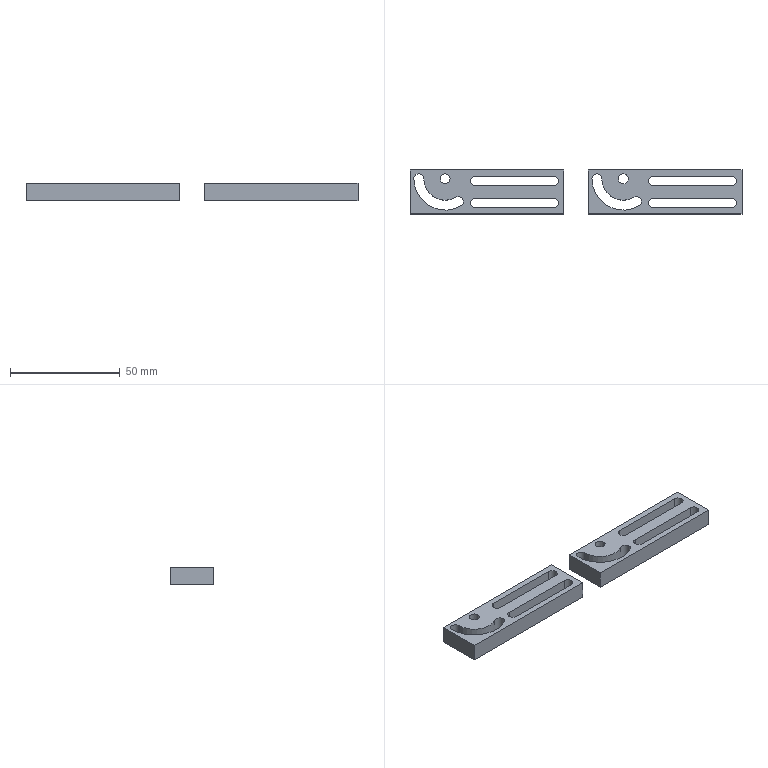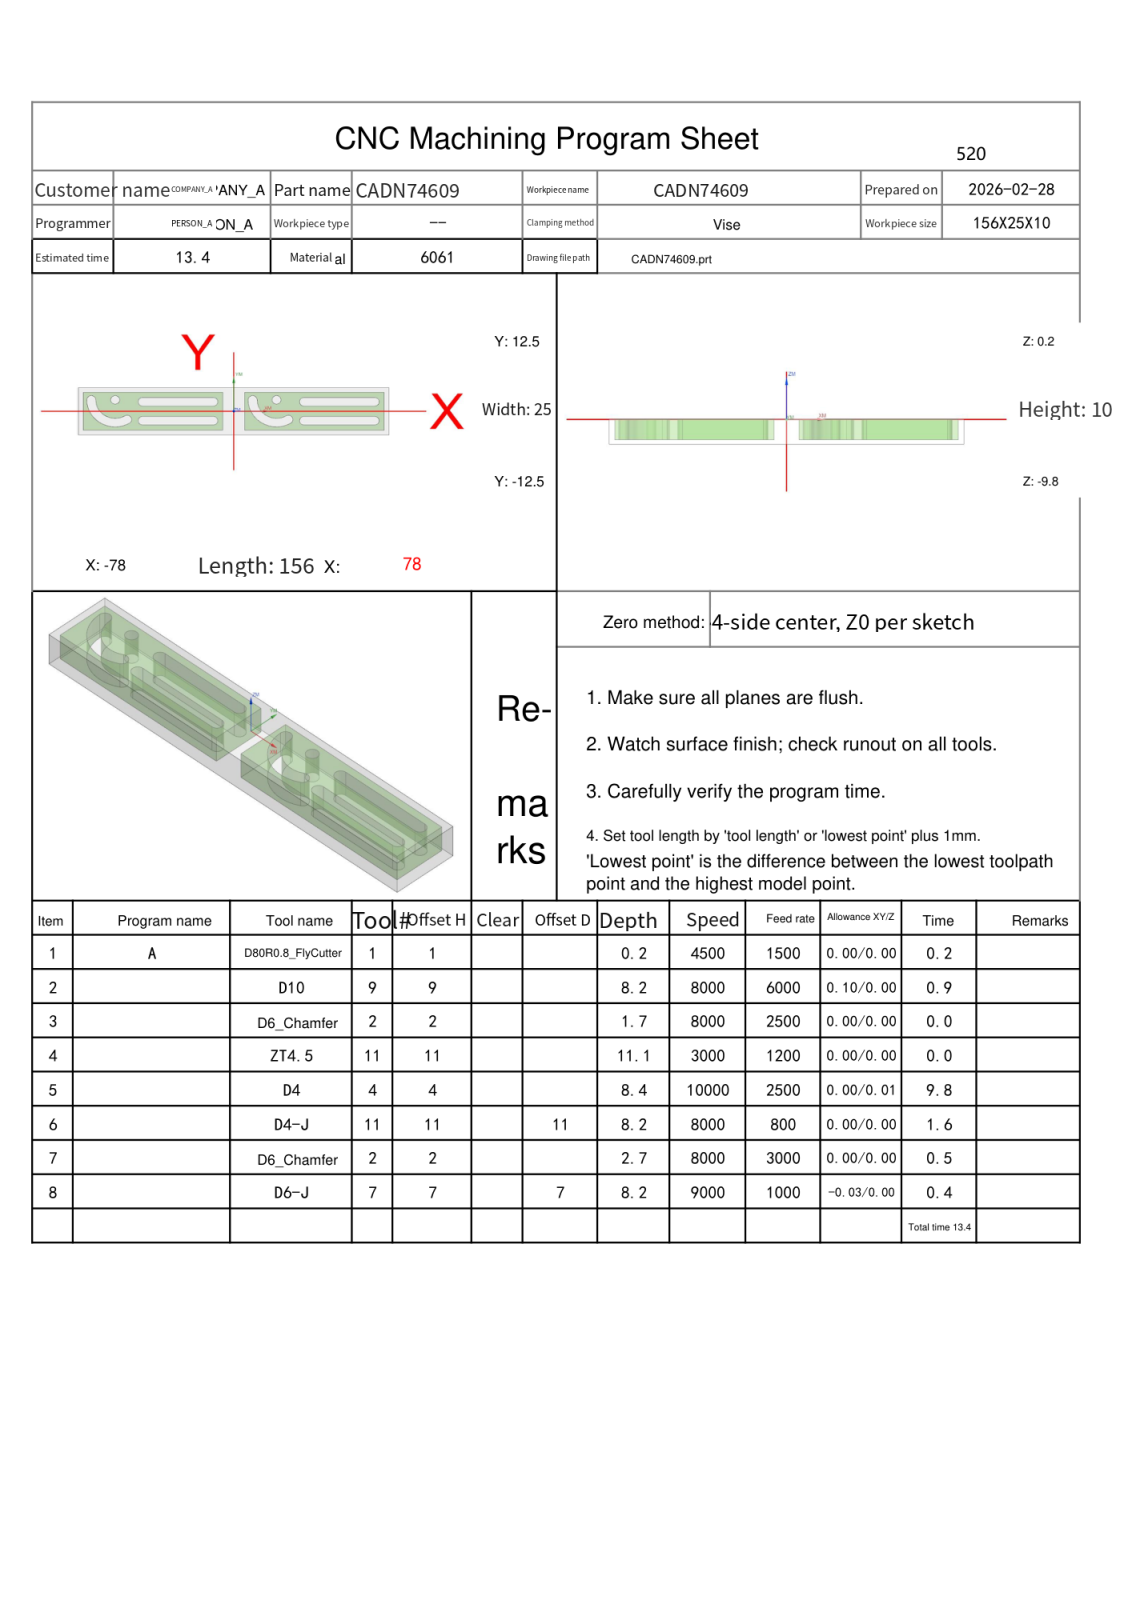NC program | NX | posted by the shop | part box 151 x 20 x 8 mm
Lines 3238 to 3746 of 3746:
N6 T11 M06
(D4-J  D=4. R=0. H=11 ce=0.00 di=0.00)
G00 G90 G54 X-28.2 Y5. M03 S8000
G43 H11 Z50.
M08
Z-3.5
G01 Z-4. F500.
G41 D11
Y4.95
G03 X-28. Y4.75 I.2 J0.0
G01 X-10.25
G03 X-10. Y5. I0.0 J.25
X-10.25 Y5.25 I-.25 J0.0
G01 X-45.75
G03 X-46. Y5. I0.0 J-.25
X-45.75 Y4.75 I.25 J0.0
G01 X-28.
X-27.5
G03 X-27.3 Y4.95 I0.0 J.2
G01 G40 Y5.
Z-3.5
G00 Z1.
X-28.2
Z-7.5
G01 Z-8.
G41 D11
Y4.95
G03 X-28. Y4.75 I.2 J0.0
G01 X-10.25
G03 X-10. Y5. I0.0 J.25
X-10.25 Y5.25 I-.25 J0.0
G01 X-45.75
G03 X-46. Y5. I0.0 J-.25
X-45.75 Y4.75 I.25 J0.0
G01 X-28.
X-27.5
G03 X-27.3 Y4.95 I0.0 J.2
G01 G40 Y5.
Z-7.5
G00 Z50.
X-27.8 Y-5.
Z-3.5
G01 Z-4.
G41 D11
Y-4.95
G03 X-28. Y-4.75 I-.2 J0.0
G01 X-45.75
G03 X-46. Y-5. I0.0 J-.25
X-45.75 Y-5.25 I.25 J0.0
G01 X-10.25
G03 X-10. Y-5. I0.0 J.25
X-10.25 Y-4.75 I-.25 J0.0
G01 X-28.
X-28.5
G03 X-28.7 Y-4.95 I0.0 J-.2
G01 G40 Y-5.
Z-3.5
G00 Z1.
X-27.8
Z-7.5
G01 Z-8.
G41 D11
Y-4.95
G03 X-28. Y-4.75 I-.2 J0.0
G01 X-45.75
G03 X-46. Y-5. I0.0 J-.25
X-45.75 Y-5.25 I.25 J0.0
G01 X-10.25
G03 X-10. Y-5. I0.0 J.25
X-10.25 Y-4.75 I-.25 J0.0
G01 X-28.
X-28.5
G03 X-28.7 Y-4.95 I0.0 J-.2
G01 G40 Y-5.
Z-7.5
G00 Z50.
X52.8 Y5.
Z-3.5
G01 Z-4.
G41 D11
Y4.95
G03 X53. Y4.75 I.2 J0.0
G01 X70.75
G03 X71. Y5. I0.0 J.25
X70.75 Y5.25 I-.25 J0.0
G01 X35.25
G03 X35. Y5. I0.0 J-.25
X35.25 Y4.75 I.25 J0.0
G01 X53.
X53.5
G03 X53.7 Y4.95 I0.0 J.2
G01 G40 Y5.
Z-3.5
G00 Z1.
X52.8
Z-7.5
G01 Z-8.
G41 D11
Y4.95
G03 X53. Y4.75 I.2 J0.0
G01 X70.75
G03 X71. Y5. I0.0 J.25
X70.75 Y5.25 I-.25 J0.0
G01 X35.25
G03 X35. Y5. I0.0 J-.25
X35.25 Y4.75 I.25 J0.0
G01 X53.
X53.5
G03 X53.7 Y4.95 I0.0 J.2
G01 G40 Y5.
Z-7.5
G00 Z50.
X53.2 Y-5.
Z-3.5
G01 Z-4.
G41 D11
Y-4.95
G03 X53. Y-4.75 I-.2 J0.0
G01 X35.25
G03 X35. Y-5. I0.0 J-.25
X35.25 Y-5.25 I.25 J0.0
G01 X70.75
G03 X71. Y-5. I0.0 J.25
X70.75 Y-4.75 I-.25 J0.0
G01 X53.
X52.5
G03 X52.3 Y-4.95 I0.0 J-.2
G01 G40 Y-5.
Z-3.5
G00 Z1.
X53.2
Z-7.5
G01 Z-8.
G41 D11
Y-4.95
G03 X53. Y-4.75 I-.2 J0.0
G01 X35.25
G03 X35. Y-5. I0.0 J-.25
X35.25 Y-5.25 I.25 J0.0
G01 X70.75
G03 X71. Y-5. I0.0 J.25
X70.75 Y-4.75 I-.25 J0.0
G01 X53.
X52.5
G03 X52.3 Y-4.95 I0.0 J-.2
G01 G40 Y-5.
Z-7.5
G00 Z50.
G00 G90 X15.328 Y-4.291 M03 S8000
Z50.
Z-3.5
G01 Z-4. F800.
G41 D11
X15.302 Y-4.336
X15.275 Y-4.436
G03 X15.375 Y-4.609 I.2 J0.0
X21.5 Y-6.25 I6.125 J10.609
X27.625 Y-4.609 I0.0 J12.25
X27.75 Y-4.392 I-.125 J.217
X27.5 Y-4.142 I-.25 J0.0
G01 X27.375 Y-4.176
G02 X21.5 Y-5.75 I-5.875 J10.176
X9.75 Y6. I0.0 J11.75
G03 X9.5 Y6.25 I-.25 J0.0
X9.25 Y6. I0.0 J-.25
X15.375 Y-4.609 I12.25 J0.0
X15.813 Y-4.85 I6.125 J10.609
G01 X15.906 Y-4.873
G03 X16.084 Y-4.764 I0.0 J.2
G01 G40 X16.107 Y-4.72
Z-3.5
G00 Z1.
X15.328 Y-4.291
Z-7.5
G01 Z-8.
G41 D11
X15.302 Y-4.336
X15.275 Y-4.436
G03 X15.375 Y-4.609 I.2 J0.0
X21.5 Y-6.25 I6.125 J10.609
X27.625 Y-4.609 I0.0 J12.25
X27.75 Y-4.392 I-.125 J.217
X27.5 Y-4.142 I-.25 J0.0
G01 X27.375 Y-4.176
G02 X21.5 Y-5.75 I-5.875 J10.176
X9.75 Y6. I0.0 J11.75
G03 X9.5 Y6.25 I-.25 J0.0
X9.25 Y6. I0.0 J-.25
X15.375 Y-4.609 I12.25 J0.0
X15.813 Y-4.85 I6.125 J10.609
G01 X15.906 Y-4.873
G03 X16.084 Y-4.764 I0.0 J.2
G01 G40 X16.107 Y-4.72
Z-7.5
G00 Z50.
X-65.672 Y-4.291
Z-3.5
G01 Z-4.
G41 D11
X-65.698 Y-4.336
X-65.725 Y-4.436
G03 X-65.625 Y-4.609 I.2 J0.0
X-59.5 Y-6.25 I6.125 J10.609
X-53.375 Y-4.609 I0.0 J12.25
X-53.25 Y-4.392 I-.125 J.217
X-53.5 Y-4.142 I-.25 J0.0
G01 X-53.625 Y-4.176
G02 X-59.5 Y-5.75 I-5.875 J10.176
X-71.25 Y6. I0.0 J11.75
G03 X-71.5 Y6.25 I-.25 J0.0
X-71.75 Y6. I0.0 J-.25
X-65.625 Y-4.609 I12.25 J0.0
X-65.187 Y-4.85 I6.125 J10.609
G01 X-65.094 Y-4.873
G03 X-64.916 Y-4.764 I0.0 J.2
G01 G40 X-64.893 Y-4.72
Z-3.5
G00 Z1.
X-65.672 Y-4.291
Z-7.5
G01 Z-8.
G41 D11
X-65.698 Y-4.336
X-65.725 Y-4.436
G03 X-65.625 Y-4.609 I.2 J0.0
X-59.5 Y-6.25 I6.125 J10.609
X-53.375 Y-4.609 I0.0 J12.25
X-53.25 Y-4.392 I-.125 J.217
X-53.5 Y-4.142 I-.25 J0.0
G01 X-53.625 Y-4.176
G02 X-59.5 Y-5.75 I-5.875 J10.176
X-71.25 Y6. I0.0 J11.75
G03 X-71.5 Y6.25 I-.25 J0.0
X-71.75 Y6. I0.0 J-.25
X-65.625 Y-4.609 I12.25 J0.0
X-65.187 Y-4.85 I6.125 J10.609
G01 X-65.094 Y-4.873
G03 X-64.916 Y-4.764 I0.0 J.2
G01 G40 X-64.893 Y-4.72
Z-7.5
G00 Z50.
G91 G28 Z0.0
M05
M09
G91 G28 Z0.0
M01
N7 T02 M06
(D6_Chamfer  D=6. R=0. H=02 ce=0.00 di=0.00)
G00 G90 G54 X-40.25 Y-12.128 M03 S8000
G43 H02 Z50.
M08
Z2.099
G01 Z-1.5 F3000.
G03 X-40.17 Y-11.828 I-.52 J.3
X-40.47 Y-11.308 I-.6 J0.0
G01 X-40.5 Y-11.3
X-75.5
G02 X-76.8 Y-10. I0.0 J1.3
G01 Y10.
G02 X-75.5 Y11.3 I1.3 J0.0
G01 X-5.5
G02 X-4.2 Y10. I0.0 J-1.3
G01 Y-10.
G02 X-5.5 Y-11.3 I-1.3 J0.0
G01 X-40.5
X-40.53 Y-11.308
G03 X-40.83 Y-11.828 I.3 J-.52
X-40.75 Y-12.128 I.6 J0.0
G01 Z2.099
G00 Z50.
X-65.809 Y-4.367
Z2.121
G01 Z-1.5
G03 X-66.09 Y-4.875 I.319 J-.508
X-65.998 Y-5.194 I.6 J0.0
G01 X-65.975 Y-5.215
G03 X-59.5 Y-6.95 I6.475 J11.215
X-53.025 Y-5.215 I0.0 J12.95
X-52.55 Y-4.392 I-.475 J.823
X-53.025 Y-3.57 I-.95 J0.0
G01 X-53.254 Y-3.475
X-53.5 Y-3.442
X-53.746 Y-3.475
X-53.975 Y-3.57
G02 X-59.5 Y-5.05 I-5.525 J9.57
X-70.55 Y6. I0.0 J11.05
G03 X-71.5 Y6.95 I-.95 J0.0
X-71.975 Y6.823 I0.0 J-.95
G01 X-72.172 Y6.672
X-72.323 Y6.475
X-72.418 Y6.246
X-72.45 Y6.
G03 X-65.975 Y-5.215 I12.95 J0.0
G01 X-65.945 Y-5.224
X-65.923 Y-5.225
G03 X-65.323 Y-4.647 I0.0 J.6
G01 Z2.121
G00 Z50.
X-28.25 Y-5.122
Z2.099
G01 Z-1.5
G03 X-28.33 Y-5.422 I.52 J-.3
X-28.03 Y-5.942 I.6 J0.0
G01 X-28. Y-5.95
X-10.25
G03 X-9.3 Y-5. I0.0 J.95
X-9.427 Y-4.525 I-.95 J0.0
G01 X-9.578 Y-4.328
X-9.775 Y-4.177
X-10.004 Y-4.082
X-10.25 Y-4.05
X-45.75
G03 X-46.7 Y-5. I0.0 J-.95
X-46.573 Y-5.475 I.95 J0.0
G01 X-46.422 Y-5.672
X-46.225 Y-5.823
X-45.996 Y-5.918
X-45.75 Y-5.95
X-28.
X-27.97 Y-5.942
G03 X-27.67 Y-5.422 I-.3 J.52
X-27.75 Y-5.122 I-.6 J0.0
G01 Z2.099
G00 Z6.
X-28.25 Y4.878
Z2.099
G01 Z-1.5
G03 X-28.33 Y4.578 I.52 J-.3
X-28.03 Y4.058 I.6 J0.0
G01 X-28. Y4.05
X-10.25
G03 X-9.3 Y5. I0.0 J.95
X-9.427 Y5.475 I-.95 J0.0
G01 X-9.578 Y5.672
X-9.775 Y5.823
X-10.004 Y5.918
X-10.25 Y5.95
X-45.75
G03 X-46.7 Y5. I0.0 J-.95
X-46.573 Y4.525 I.95 J0.0
G01 X-46.422 Y4.328
X-46.225 Y4.177
X-45.996 Y4.082
X-45.75 Y4.05
X-28.
X-27.97 Y4.058
G03 X-27.67 Y4.578 I-.3 J.52
X-27.75 Y4.878 I-.6 J0.0
G01 Z2.099
G00 Z50.
X40.25 Y12.128
Z2.099
G01 Z-1.5
G03 X40.17 Y11.828 I.52 J-.3
X40.47 Y11.308 I.6 J0.0
G01 X40.5 Y11.3
X75.5
G02 X76.8 Y10. I0.0 J-1.3
G01 Y-10.
G02 X75.5 Y-11.3 I-1.3 J0.0
G01 X5.5
G02 X4.2 Y-10. I0.0 J1.3
G01 Y10.
G02 X5.5 Y11.3 I1.3 J0.0
G01 X40.5
X40.53 Y11.308
G03 X40.83 Y11.828 I-.3 J.52
X40.75 Y12.128 I-.6 J0.0
G01 Z2.099
G00 Z50.
X15.191 Y-4.367
Z2.121
G01 Z-1.5
G03 X14.91 Y-4.875 I.319 J-.508
X15.002 Y-5.194 I.6 J0.0
G01 X15.025 Y-5.215
G03 X21.5 Y-6.95 I6.475 J11.215
X27.975 Y-5.215 I0.0 J12.95
X28.45 Y-4.392 I-.475 J.823
X27.975 Y-3.57 I-.95 J0.0
G01 X27.746 Y-3.475
X27.5 Y-3.442
X27.254 Y-3.475
X27.025 Y-3.57
G02 X21.5 Y-5.05 I-5.525 J9.57
X10.45 Y6. I0.0 J11.05
G03 X9.5 Y6.95 I-.95 J0.0
X9.025 Y6.823 I0.0 J-.95
G01 X8.828 Y6.672
X8.677 Y6.475
X8.582 Y6.246
X8.55 Y6.
G03 X15.025 Y-5.215 I12.95 J0.0
G01 X15.055 Y-5.224
X15.077 Y-5.225
G03 X15.677 Y-4.647 I0.0 J.6
G01 Z2.121
G00 Z50.
X52.75 Y-5.122
Z2.099
G01 Z-1.5
G03 X52.67 Y-5.422 I.52 J-.3
X52.97 Y-5.942 I.6 J0.0
G01 X53. Y-5.95
X70.75
G03 X71.7 Y-5. I0.0 J.95
X71.573 Y-4.525 I-.95 J0.0
G01 X71.422 Y-4.328
X71.225 Y-4.177
X70.996 Y-4.082
X70.75 Y-4.05
X35.25
G03 X34.3 Y-5. I0.0 J-.95
X34.427 Y-5.475 I.95 J0.0
G01 X34.578 Y-5.672
X34.775 Y-5.823
X35.004 Y-5.918
X35.25 Y-5.95
X53.
X53.03 Y-5.942
G03 X53.33 Y-5.422 I-.3 J.52
X53.25 Y-5.122 I-.6 J0.0
G01 Z2.099
G00 Z6.
X52.75 Y4.878
Z2.099
G01 Z-1.5
G03 X52.67 Y4.578 I.52 J-.3
X52.97 Y4.058 I.6 J0.0
G01 X53. Y4.05
X70.75
G03 X71.7 Y5. I0.0 J.95
X71.573 Y5.475 I-.95 J0.0
G01 X71.422 Y5.672
X71.225 Y5.823
X70.996 Y5.918
X70.75 Y5.95
X35.25
G03 X34.3 Y5. I0.0 J-.95
X34.427 Y4.525 I.95 J0.0
G01 X34.578 Y4.328
X34.775 Y4.177
X35.004 Y4.082
X35.25 Y4.05
X53.
X53.03 Y4.058
G03 X53.33 Y4.578 I-.3 J.52
X53.25 Y4.878 I-.6 J0.0
G01 Z2.099
G00 Z50.
G00 G90 X-59.5 Y6. M03 S8000
Z50.
G98 G81 X-59.5 Y6. Z-2.55 R3. F150.
X21.5
G80
G00 Z50.
G91 G28 Z0.0
M05
M09
G91 G28 Z0.0
M01
N8 T07 M06
(D6-J  D=6. R=0. H=07 ce=-0.03 di=0.00)
G00 G90 G54 X-4.483 Y-14.048 M03 S9000
G43 H07 Z50.
M08
Z-7.5
G01 Z-8. F1000.
G41 D07
X-4.508 Y-13.849
G03 X-5.5 Y-12.975 I-.992 J-.126
G01 X-75.5
G02 X-78.475 Y-10. I0.0 J2.975
G01 Y10.
G02 X-75.5 Y12.975 I2.975 J0.0
G01 X-5.5
G02 X-2.525 Y10. I0.0 J-2.975
G01 Y-10.
G02 X-5.5 Y-12.975 I-2.975 J0.0
G01 X-6.
G03 X-7. Y-13.975 I0.0 J-1.
G01 G40 Y-14.175
Z-7.5
G00 Z50.
X76.517 Y-14.048
Z-7.5
G01 Z-8.
G41 D07
X76.492 Y-13.849
G03 X75.5 Y-12.975 I-.992 J-.126
G01 X5.5
G02 X2.525 Y-10. I0.0 J2.975
G01 Y10.
G02 X5.5 Y12.975 I2.975 J0.0
G01 X75.5
G02 X78.475 Y10. I0.0 J-2.975
G01 Y-10.
G02 X75.5 Y-12.975 I-2.975 J0.0
G01 X75.
G03 X74. Y-13.975 I0.0 J-1.
G01 G40 Y-14.175
Z-7.5
G00 Z50.
M05
M09
G91 G28 Z0.0
G91 G28 Y0.0
M30
%